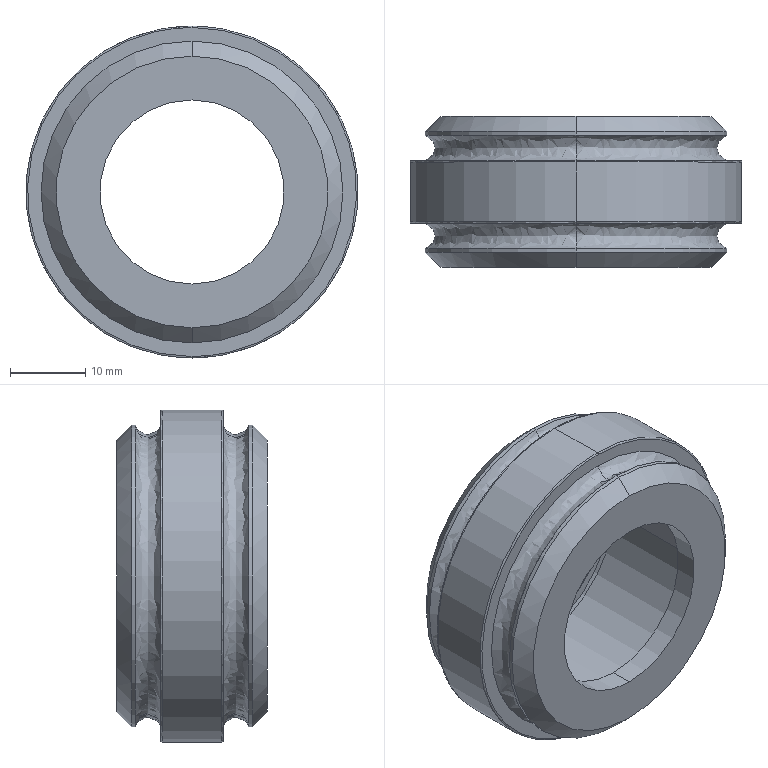Part | SolidWorks | features BaseBody 1 | 1 solid | 33 faces | box 44 x 20 x 44 mm | volume 14039 mm3 | cylinder 14 | spline 8 | plane 7 | cone 4 | commonest cylinder face diameters 28 x4 40 x4 24.4 x2 30.1 x2 44 x2
STEP:
#1=CARTESIAN_POINT('',(0.,2.5,-20.));
#2=VERTEX_POINT('',#1);
#3=CARTESIAN_POINT('',(0.,2.5,20.));
#4=VERTEX_POINT('',#3);
#5=CARTESIAN_POINT('',(0.,2.5,0.));
#6=DIRECTION('',(0.,-1.,0.));
#7=DIRECTION('',(0.,0.,1.));
#8=AXIS2_PLACEMENT_3D('',#5,#6,#7);
#9=CIRCLE('',#8,20.);
#10=EDGE_CURVE('',#2,#4,#9,.T.);
#11=ORIENTED_EDGE('',*,*,#10,.F.);
#12=CARTESIAN_POINT('',(0.,5.85,-20.));
#13=VERTEX_POINT('',#12);
#14=CARTESIAN_POINT('',(0.,4.175,-20.407));
#15=DIRECTION('',(-1.,0.,0.));
#16=DIRECTION('',(0.,0.,-1.));
#17=AXIS2_PLACEMENT_3D('',#14,#15,#16);
#18=CIRCLE('',#17,1.724);
#19=EDGE_CURVE('',#2,#13,#18,.T.);
#20=ORIENTED_EDGE('',*,*,#19,.T.);
#21=CARTESIAN_POINT('',(0.,5.85,20.));
#22=VERTEX_POINT('',#21);
#23=CARTESIAN_POINT('',(0.,5.85,0.));
#24=DIRECTION('',(0.,1.,0.));
#25=DIRECTION('',(0.,0.,1.));
#26=AXIS2_PLACEMENT_3D('',#23,#24,#25);
#27=CIRCLE('',#26,20.);
#28=EDGE_CURVE('',#22,#13,#27,.T.);
#29=ORIENTED_EDGE('',*,*,#28,.F.);
#30=CARTESIAN_POINT('',(0.,4.175,20.407));
#31=DIRECTION('',(1.,0.,0.));
#32=DIRECTION('',(0.,0.,1.));
#33=AXIS2_PLACEMENT_3D('',#30,#31,#32);
#34=CIRCLE('',#33,1.724);
#35=EDGE_CURVE('',#4,#22,#34,.T.);
#36=ORIENTED_EDGE('',*,*,#35,.F.);
#37=EDGE_LOOP('',(#11,#20,#29,#36));
#38=FACE_OUTER_BOUND('',#37,.T.);
#39=CARTESIAN_POINT('',(0.,2.5,20.));
#40=CARTESIAN_POINT('',(40.,2.5,20.));
#41=CARTESIAN_POINT('',(40.,2.5,-20.));
#42=CARTESIAN_POINT('',(0.,2.5,-20.));
#43=CARTESIAN_POINT('',(0.,3.037,17.789));
#44=CARTESIAN_POINT('',(35.578,3.037,17.789));
#45=CARTESIAN_POINT('',(35.578,3.037,-17.789));
#46=CARTESIAN_POINT('',(0.,3.037,-17.789));
#47=CARTESIAN_POINT('',(0.,5.313,17.789));
#48=CARTESIAN_POINT('',(35.578,5.313,17.789));
#49=CARTESIAN_POINT('',(35.578,5.313,-17.789));
#50=CARTESIAN_POINT('',(0.,5.313,-17.789));
#51=CARTESIAN_POINT('',(0.,5.85,20.));
#52=CARTESIAN_POINT('',(40.,5.85,20.));
#53=CARTESIAN_POINT('',(40.,5.85,-20.));
#54=CARTESIAN_POINT('',(0.,5.85,-20.));
#55=(BOUNDED_SURFACE()B_SPLINE_SURFACE(3,3,((#39,#40,#41,#42),(#43,#44,#45,#46),(#47,#48,#49,#50),(#51,#52,#53,#54)),.UNSPECIFIED.,.F.,.F.,.F.)B_SPLINE_SURFACE_WITH_KNOTS((4,4),(4,4),(0.,1.),(0.,1.),.UNSPECIFIED.)GEOMETRIC_REPRESENTATION_ITEM()RATIONAL_B_SPLINE_SURFACE(((1.,0.3333,0.3333,1.),(0.4907,0.1636,0.1636,0.4907),(0.4907,0.1636,0.1636,0.4907),(1.,0.3333,0.3333,1.)))REPRESENTATION_ITEM('')SURFACE());
#56=ADVANCED_FACE('',(#38),#55,.F.);
#57=CARTESIAN_POINT('',(0.,14.15,-20.));
#58=VERTEX_POINT('',#57);
#59=CARTESIAN_POINT('',(0.,14.15,20.));
#60=VERTEX_POINT('',#59);
#61=CARTESIAN_POINT('',(0.,14.15,0.));
#62=DIRECTION('',(0.,-1.,0.));
#63=DIRECTION('',(0.,0.,1.));
#64=AXIS2_PLACEMENT_3D('',#61,#62,#63);
#65=CIRCLE('',#64,20.);
#66=EDGE_CURVE('',#58,#60,#65,.T.);
#67=ORIENTED_EDGE('',*,*,#66,.F.);
#68=CARTESIAN_POINT('',(0.,17.5,-20.));
#69=VERTEX_POINT('',#68);
#70=CARTESIAN_POINT('',(0.,15.825,-20.407));
#71=DIRECTION('',(-1.,0.,0.));
#72=DIRECTION('',(0.,0.,-1.));
#73=AXIS2_PLACEMENT_3D('',#70,#71,#72);
#74=CIRCLE('',#73,1.724);
#75=EDGE_CURVE('',#58,#69,#74,.T.);
#76=ORIENTED_EDGE('',*,*,#75,.T.);
#77=CARTESIAN_POINT('',(0.,17.5,20.));
#78=VERTEX_POINT('',#77);
#79=CARTESIAN_POINT('',(0.,17.5,0.));
#80=DIRECTION('',(0.,1.,0.));
#81=DIRECTION('',(0.,0.,1.));
#82=AXIS2_PLACEMENT_3D('',#79,#80,#81);
#83=CIRCLE('',#82,20.);
#84=EDGE_CURVE('',#78,#69,#83,.T.);
#85=ORIENTED_EDGE('',*,*,#84,.F.);
#86=CARTESIAN_POINT('',(0.,15.825,20.407));
#87=DIRECTION('',(1.,0.,0.));
#88=DIRECTION('',(0.,0.,1.));
#89=AXIS2_PLACEMENT_3D('',#86,#87,#88);
#90=CIRCLE('',#89,1.724);
#91=EDGE_CURVE('',#60,#78,#90,.T.);
#92=ORIENTED_EDGE('',*,*,#91,.F.);
#93=EDGE_LOOP('',(#67,#76,#85,#92));
#94=FACE_OUTER_BOUND('',#93,.T.);
#95=CARTESIAN_POINT('',(0.,14.15,20.));
#96=CARTESIAN_POINT('',(40.,14.15,20.));
#97=CARTESIAN_POINT('',(40.,14.15,-20.));
#98=CARTESIAN_POINT('',(0.,14.15,-20.));
#99=CARTESIAN_POINT('',(0.,14.687,17.789));
#100=CARTESIAN_POINT('',(35.578,14.687,17.789));
#101=CARTESIAN_POINT('',(35.578,14.687,-17.789));
#102=CARTESIAN_POINT('',(0.,14.687,-17.789));
#103=CARTESIAN_POINT('',(0.,16.963,17.789));
#104=CARTESIAN_POINT('',(35.578,16.963,17.789));
#105=CARTESIAN_POINT('',(35.578,16.963,-17.789));
#106=CARTESIAN_POINT('',(0.,16.963,-17.789));
#107=CARTESIAN_POINT('',(0.,17.5,20.));
#108=CARTESIAN_POINT('',(40.,17.5,20.));
#109=CARTESIAN_POINT('',(40.,17.5,-20.));
#110=CARTESIAN_POINT('',(0.,17.5,-20.));
#111=(BOUNDED_SURFACE()B_SPLINE_SURFACE(3,3,((#95,#96,#97,#98),(#99,#100,#101,#102),(#103,#104,#105,#106),(#107,#108,#109,#110)),.UNSPECIFIED.,.F.,.F.,.T.)B_SPLINE_SURFACE_WITH_KNOTS((4,4),(4,4),(0.,1.),(0.,1.),.UNSPECIFIED.)GEOMETRIC_REPRESENTATION_ITEM()RATIONAL_B_SPLINE_SURFACE(((1.,0.3333,0.3333,1.),(0.4907,0.1636,0.1636,0.4907),(0.4907,0.1636,0.1636,0.4907),(1.,0.3333,0.3333,1.)))REPRESENTATION_ITEM('')SURFACE());
#112=ADVANCED_FACE('',(#94),#111,.F.);
#113=CARTESIAN_POINT('',(0.,6.05,22.));
#114=VERTEX_POINT('',#113);
#115=CARTESIAN_POINT('',(0.,6.05,-22.));
#116=VERTEX_POINT('',#115);
#117=CARTESIAN_POINT('',(0.,6.05,0.));
#118=DIRECTION('',(0.,-1.,0.));
#119=DIRECTION('',(0.,0.,1.));
#120=AXIS2_PLACEMENT_3D('',#117,#118,#119);
#121=CIRCLE('',#120,22.);
#122=EDGE_CURVE('',#114,#116,#121,.T.);
#123=ORIENTED_EDGE('',*,*,#122,.T.);
#124=CARTESIAN_POINT('',(0.,5.85,-21.8));
#125=VERTEX_POINT('',#124);
#126=CARTESIAN_POINT('',(0.,6.05,-21.8));
#127=DIRECTION('',(-1.,0.,0.));
#128=DIRECTION('',(0.,0.,-1.));
#129=AXIS2_PLACEMENT_3D('',#126,#127,#128);
#130=CIRCLE('',#129,0.2);
#131=EDGE_CURVE('',#116,#125,#130,.T.);
#132=ORIENTED_EDGE('',*,*,#131,.T.);
#133=CARTESIAN_POINT('',(0.,5.85,21.8));
#134=VERTEX_POINT('',#133);
#135=CARTESIAN_POINT('',(0.,5.85,-21.8));
#136=CARTESIAN_POINT('',(-43.6,5.85,-21.8));
#137=CARTESIAN_POINT('',(-43.6,5.85,21.8));
#138=CARTESIAN_POINT('',(0.,5.85,21.8));
#139=(BOUNDED_CURVE()B_SPLINE_CURVE(3,(#135,#136,#137,#138),.UNSPECIFIED.,.F.,.F.)B_SPLINE_CURVE_WITH_KNOTS((4,4),(0.,1.),.UNSPECIFIED.)CURVE()GEOMETRIC_REPRESENTATION_ITEM()RATIONAL_B_SPLINE_CURVE((1.,0.3333,0.3333,1.))REPRESENTATION_ITEM(''));
#140=EDGE_CURVE('',#125,#134,#139,.T.);
#141=ORIENTED_EDGE('',*,*,#140,.T.);
#142=CARTESIAN_POINT('',(0.,6.05,21.8));
#143=DIRECTION('',(1.,0.,0.));
#144=DIRECTION('',(0.,0.,1.));
#145=AXIS2_PLACEMENT_3D('',#142,#143,#144);
#146=CIRCLE('',#145,0.2);
#147=EDGE_CURVE('',#114,#134,#146,.T.);
#148=ORIENTED_EDGE('',*,*,#147,.F.);
#149=EDGE_LOOP('',(#123,#132,#141,#148));
#150=FACE_OUTER_BOUND('',#149,.T.);
#151=CARTESIAN_POINT('',(0.,6.05,-22.));
#152=CARTESIAN_POINT('',(-44.,6.05,-22.));
#153=CARTESIAN_POINT('',(-44.,6.05,22.));
#154=CARTESIAN_POINT('',(0.,6.05,22.));
#155=CARTESIAN_POINT('',(0.,5.933,-22.));
#156=CARTESIAN_POINT('',(-44.,5.933,-22.));
#157=CARTESIAN_POINT('',(-44.,5.933,22.));
#158=CARTESIAN_POINT('',(0.,5.933,22.));
#159=CARTESIAN_POINT('',(0.,5.85,-21.917));
#160=CARTESIAN_POINT('',(-43.834,5.85,-21.917));
#161=CARTESIAN_POINT('',(-43.834,5.85,21.917));
#162=CARTESIAN_POINT('',(0.,5.85,21.917));
#163=CARTESIAN_POINT('',(0.,5.85,-21.8));
#164=CARTESIAN_POINT('',(-43.6,5.85,-21.8));
#165=CARTESIAN_POINT('',(-43.6,5.85,21.8));
#166=CARTESIAN_POINT('',(0.,5.85,21.8));
#167=(BOUNDED_SURFACE()B_SPLINE_SURFACE(3,3,((#151,#152,#153,#154),(#155,#156,#157,#158),(#159,#160,#161,#162),(#163,#164,#165,#166)),.UNSPECIFIED.,.F.,.F.,.F.)B_SPLINE_SURFACE_WITH_KNOTS((4,4),(4,4),(0.,1.),(0.,1.),.UNSPECIFIED.)GEOMETRIC_REPRESENTATION_ITEM()RATIONAL_B_SPLINE_SURFACE(((1.,0.3333,0.3333,1.),(0.8047,0.2682,0.2682,0.8047),(0.8047,0.2682,0.2682,0.8047),(1.,0.3333,0.3333,1.)))REPRESENTATION_ITEM('')SURFACE());
#168=ADVANCED_FACE('',(#150),#167,.T.);
#169=CARTESIAN_POINT('',(0.,13.95,22.));
#170=VERTEX_POINT('',#169);
#171=CARTESIAN_POINT('',(0.,13.95,-22.));
#172=VERTEX_POINT('',#171);
#173=CARTESIAN_POINT('',(0.,13.95,0.));
#174=DIRECTION('',(0.,-1.,0.));
#175=DIRECTION('',(0.,0.,1.));
#176=AXIS2_PLACEMENT_3D('',#173,#174,#175);
#177=CIRCLE('',#176,22.);
#178=EDGE_CURVE('',#170,#172,#177,.T.);
#179=ORIENTED_EDGE('',*,*,#178,.F.);
#180=CARTESIAN_POINT('',(0.,14.15,21.8));
#181=VERTEX_POINT('',#180);
#182=CARTESIAN_POINT('',(0.,13.95,21.8));
#183=DIRECTION('',(-1.,0.,0.));
#184=DIRECTION('',(0.,0.,1.));
#185=AXIS2_PLACEMENT_3D('',#182,#183,#184);
#186=CIRCLE('',#185,0.2);
#187=EDGE_CURVE('',#170,#181,#186,.T.);
#188=ORIENTED_EDGE('',*,*,#187,.T.);
#189=CARTESIAN_POINT('',(0.,14.15,-21.8));
#190=VERTEX_POINT('',#189);
#191=CARTESIAN_POINT('',(0.,14.15,21.8));
#192=CARTESIAN_POINT('',(-43.6,14.15,21.8));
#193=CARTESIAN_POINT('',(-43.6,14.15,-21.8));
#194=CARTESIAN_POINT('',(0.,14.15,-21.8));
#195=(BOUNDED_CURVE()B_SPLINE_CURVE(3,(#191,#192,#193,#194),.UNSPECIFIED.,.F.,.F.)B_SPLINE_CURVE_WITH_KNOTS((4,4),(0.,1.),.UNSPECIFIED.)CURVE()GEOMETRIC_REPRESENTATION_ITEM()RATIONAL_B_SPLINE_CURVE((1.,0.3333,0.3333,1.))REPRESENTATION_ITEM(''));
#196=EDGE_CURVE('',#181,#190,#195,.T.);
#197=ORIENTED_EDGE('',*,*,#196,.T.);
#198=CARTESIAN_POINT('',(0.,13.95,-21.8));
#199=DIRECTION('',(1.,0.,0.));
#200=DIRECTION('',(0.,0.,-1.));
#201=AXIS2_PLACEMENT_3D('',#198,#199,#200);
#202=CIRCLE('',#201,0.2);
#203=EDGE_CURVE('',#172,#190,#202,.T.);
#204=ORIENTED_EDGE('',*,*,#203,.F.);
#205=EDGE_LOOP('',(#179,#188,#197,#204));
#206=FACE_OUTER_BOUND('',#205,.T.);
#207=CARTESIAN_POINT('',(0.,13.95,22.));
#208=CARTESIAN_POINT('',(-44.,13.95,22.));
#209=CARTESIAN_POINT('',(-44.,13.95,-22.));
#210=CARTESIAN_POINT('',(0.,13.95,-22.));
#211=CARTESIAN_POINT('',(0.,14.067,22.));
#212=CARTESIAN_POINT('',(-44.,14.067,22.));
#213=CARTESIAN_POINT('',(-44.,14.067,-22.));
#214=CARTESIAN_POINT('',(0.,14.067,-22.));
#215=CARTESIAN_POINT('',(0.,14.15,21.917));
#216=CARTESIAN_POINT('',(-43.834,14.15,21.917));
#217=CARTESIAN_POINT('',(-43.834,14.15,-21.917));
#218=CARTESIAN_POINT('',(0.,14.15,-21.917));
#219=CARTESIAN_POINT('',(0.,14.15,21.8));
#220=CARTESIAN_POINT('',(-43.6,14.15,21.8));
#221=CARTESIAN_POINT('',(-43.6,14.15,-21.8));
#222=CARTESIAN_POINT('',(0.,14.15,-21.8));
#223=(BOUNDED_SURFACE()B_SPLINE_SURFACE(3,3,((#207,#208,#209,#210),(#211,#212,#213,#214),(#215,#216,#217,#218),(#219,#220,#221,#222)),.UNSPECIFIED.,.F.,.F.,.T.)B_SPLINE_SURFACE_WITH_KNOTS((4,4),(4,4),(0.,1.),(0.,1.),.UNSPECIFIED.)GEOMETRIC_REPRESENTATION_ITEM()RATIONAL_B_SPLINE_SURFACE(((1.,0.3333,0.3333,1.),(0.8047,0.2682,0.2682,0.8047),(0.8047,0.2682,0.2682,0.8047),(1.,0.3333,0.3333,1.)))REPRESENTATION_ITEM('')SURFACE());
#224=ADVANCED_FACE('',(#206),#223,.T.);
#225=CARTESIAN_POINT('',(14.,3.,0.));
#226=VERTEX_POINT('',#225);
#227=CARTESIAN_POINT('',(-14.,3.,0.));
#228=VERTEX_POINT('',#227);
#229=CARTESIAN_POINT('',(0.,3.,0.));
#230=DIRECTION('',(0.,1.,0.));
#231=DIRECTION('',(-1.,0.,0.));
#232=AXIS2_PLACEMENT_3D('',#229,#230,#231);
#233=CIRCLE('',#232,14.);
#234=EDGE_CURVE('',#226,#228,#233,.T.);
#235=ORIENTED_EDGE('',*,*,#234,.F.);
#236=CARTESIAN_POINT('',(14.,17.,0.));
#237=VERTEX_POINT('',#236);
#238=CARTESIAN_POINT('',(14.,3.,0.));
#239=DIRECTION('',(0.,1.,0.));
#240=VECTOR('',#239,1000.);
#241=LINE('',#238,#240);
#242=EDGE_CURVE('',#226,#237,#241,.T.);
#243=ORIENTED_EDGE('',*,*,#242,.T.);
#244=CARTESIAN_POINT('',(-14.,17.,0.));
#245=VERTEX_POINT('',#244);
#246=CARTESIAN_POINT('',(0.,17.,0.));
#247=DIRECTION('',(0.,-1.,0.));
#248=DIRECTION('',(-1.,0.,0.));
#249=AXIS2_PLACEMENT_3D('',#246,#247,#248);
#250=CIRCLE('',#249,14.);
#251=EDGE_CURVE('',#245,#237,#250,.T.);
#252=ORIENTED_EDGE('',*,*,#251,.F.);
#253=CARTESIAN_POINT('',(-14.,3.,0.));
#254=DIRECTION('',(0.,1.,0.));
#255=VECTOR('',#254,1000.);
#256=LINE('',#253,#255);
#257=EDGE_CURVE('',#228,#245,#256,.T.);
#258=ORIENTED_EDGE('',*,*,#257,.F.);
#259=EDGE_LOOP('',(#235,#243,#252,#258));
#260=FACE_OUTER_BOUND('',#259,.T.);
#261=CARTESIAN_POINT('',(0.,3.,0.));
#262=DIRECTION('',(0.,1.,0.));
#263=DIRECTION('',(-1.,0.,0.));
#264=AXIS2_PLACEMENT_3D('',#261,#262,#263);
#265=CYLINDRICAL_SURFACE('',#264,14.);
#266=ADVANCED_FACE('',(#260),#265,.F.);
#267=CARTESIAN_POINT('',(0.,3.,12.2));
#268=VERTEX_POINT('',#267);
#269=CARTESIAN_POINT('',(0.,3.,-12.2));
#270=VERTEX_POINT('',#269);
#271=CARTESIAN_POINT('',(0.,3.,0.));
#272=DIRECTION('',(0.,-1.,0.));
#273=DIRECTION('',(0.,0.,-1.));
#274=AXIS2_PLACEMENT_3D('',#271,#272,#273);
#275=CIRCLE('',#274,12.2);
#276=EDGE_CURVE('',#268,#270,#275,.T.);
#277=ORIENTED_EDGE('',*,*,#276,.F.);
#278=CARTESIAN_POINT('',(0.,0.,12.2));
#279=VERTEX_POINT('',#278);
#280=CARTESIAN_POINT('',(0.,20.,12.2));
#281=DIRECTION('',(0.,-1.,0.));
#282=VECTOR('',#281,1000.);
#283=LINE('',#280,#282);
#284=EDGE_CURVE('',#268,#279,#283,.T.);
#285=ORIENTED_EDGE('',*,*,#284,.T.);
#286=CARTESIAN_POINT('',(0.,0.,-12.2));
#287=VERTEX_POINT('',#286);
#288=CARTESIAN_POINT('',(0.,0.,0.));
#289=DIRECTION('',(0.,1.,0.));
#290=DIRECTION('',(0.,0.,-1.));
#291=AXIS2_PLACEMENT_3D('',#288,#289,#290);
#292=CIRCLE('',#291,12.2);
#293=EDGE_CURVE('',#287,#279,#292,.T.);
#294=ORIENTED_EDGE('',*,*,#293,.F.);
#295=CARTESIAN_POINT('',(0.,20.,-12.2));
#296=DIRECTION('',(0.,-1.,0.));
#297=VECTOR('',#296,1000.);
#298=LINE('',#295,#297);
#299=EDGE_CURVE('',#270,#287,#298,.T.);
#300=ORIENTED_EDGE('',*,*,#299,.F.);
#301=EDGE_LOOP('',(#277,#285,#294,#300));
#302=FACE_OUTER_BOUND('',#301,.T.);
#303=CARTESIAN_POINT('',(0.,20.,0.));
#304=DIRECTION('',(0.,-1.,0.));
#305=DIRECTION('',(0.,0.,-1.));
#306=AXIS2_PLACEMENT_3D('',#303,#304,#305);
#307=CYLINDRICAL_SURFACE('',#306,12.2);
#308=ADVANCED_FACE('',(#302),#307,.F.);
#309=CARTESIAN_POINT('',(-15.05,18.3,0.));
#310=VERTEX_POINT('',#309);
#311=CARTESIAN_POINT('',(15.05,18.3,0.));
#312=VERTEX_POINT('',#311);
#313=CARTESIAN_POINT('',(0.,18.3,0.));
#314=DIRECTION('',(0.,-1.,0.));
#315=DIRECTION('',(1.,0.,0.));
#316=AXIS2_PLACEMENT_3D('',#313,#314,#315);
#317=CIRCLE('',#316,15.05);
#318=EDGE_CURVE('',#310,#312,#317,.T.);
#319=ORIENTED_EDGE('',*,*,#318,.F.);
#320=CARTESIAN_POINT('',(-15.05,17.,0.));
#321=VERTEX_POINT('',#320);
#322=CARTESIAN_POINT('',(-15.05,18.3,0.));
#323=DIRECTION('',(0.,-1.,0.));
#324=VECTOR('',#323,1000.);
#325=LINE('',#322,#324);
#326=EDGE_CURVE('',#310,#321,#325,.T.);
#327=ORIENTED_EDGE('',*,*,#326,.T.);
#328=CARTESIAN_POINT('',(15.05,17.,0.));
#329=VERTEX_POINT('',#328);
#330=CARTESIAN_POINT('',(0.,17.,0.));
#331=DIRECTION('',(0.,1.,0.));
#332=DIRECTION('',(1.,0.,0.));
#333=AXIS2_PLACEMENT_3D('',#330,#331,#332);
#334=CIRCLE('',#333,15.05);
#335=EDGE_CURVE('',#329,#321,#334,.T.);
#336=ORIENTED_EDGE('',*,*,#335,.F.);
#337=CARTESIAN_POINT('',(15.05,18.3,0.));
#338=DIRECTION('',(0.,-1.,0.));
#339=VECTOR('',#338,1000.);
#340=LINE('',#337,#339);
#341=EDGE_CURVE('',#312,#329,#340,.T.);
#342=ORIENTED_EDGE('',*,*,#341,.F.);
#343=EDGE_LOOP('',(#319,#327,#336,#342));
#344=FACE_OUTER_BOUND('',#343,.T.);
#345=CARTESIAN_POINT('',(0.,18.3,0.));
#346=DIRECTION('',(0.,-1.,0.));
#347=DIRECTION('',(1.,0.,0.));
#348=AXIS2_PLACEMENT_3D('',#345,#346,#347);
#349=CYLINDRICAL_SURFACE('',#348,15.05);
#350=ADVANCED_FACE('',(#344),#349,.F.);
#351=CARTESIAN_POINT('',(0.,0.,18.));
#352=VERTEX_POINT('',#351);
#353=CARTESIAN_POINT('',(0.,0.,-18.));
#354=VERTEX_POINT('',#353);
#355=CARTESIAN_POINT('',(0.,0.,0.));
#356=DIRECTION('',(0.,1.,0.));
#357=DIRECTION('',(0.,0.,1.));
#358=AXIS2_PLACEMENT_3D('',#355,#356,#357);
#359=CIRCLE('',#358,18.);
#360=EDGE_CURVE('',#352,#354,#359,.T.);
#361=ORIENTED_EDGE('',*,*,#360,.T.);
#362=CARTESIAN_POINT('',(0.,2.,-20.));
#363=VERTEX_POINT('',#362);
#364=CARTESIAN_POINT('',(0.,2.,-20.));
#365=DIRECTION('',(0.,0.7071,-0.7071));
#366=VECTOR('',#365,1000.);
#367=LINE('',#364,#366);
#368=EDGE_CURVE('',#354,#363,#367,.T.);
#369=ORIENTED_EDGE('',*,*,#368,.T.);
#370=CARTESIAN_POINT('',(0.,2.,20.));
#371=VERTEX_POINT('',#370);
#372=CARTESIAN_POINT('',(0.,2.,0.));
#373=DIRECTION('',(0.,-1.,0.));
#374=DIRECTION('',(0.,0.,1.));
#375=AXIS2_PLACEMENT_3D('',#372,#373,#374);
#376=CIRCLE('',#375,20.);
#377=EDGE_CURVE('',#363,#371,#376,.T.);
#378=ORIENTED_EDGE('',*,*,#377,.T.);
#379=CARTESIAN_POINT('',(0.,2.,20.));
#380=DIRECTION('',(0.,0.7071,0.7071));
#381=VECTOR('',#380,1000.);
#382=LINE('',#379,#381);
#383=EDGE_CURVE('',#352,#371,#382,.T.);
#384=ORIENTED_EDGE('',*,*,#383,.F.);
#385=EDGE_LOOP('',(#361,#369,#378,#384));
#386=FACE_OUTER_BOUND('',#385,.T.);
#387=CARTESIAN_POINT('',(0.,2.,0.));
#388=DIRECTION('',(0.,1.,0.));
#389=DIRECTION('',(0.,0.,1.));
#390=AXIS2_PLACEMENT_3D('',#387,#388,#389);
#391=CONICAL_SURFACE('',#390,20.,0.7854);
#392=ADVANCED_FACE('',(#386),#391,.T.);
#393=CARTESIAN_POINT('',(-14.,18.3,0.));
#394=VERTEX_POINT('',#393);
#395=CARTESIAN_POINT('',(14.,18.3,0.));
#396=VERTEX_POINT('',#395);
#397=CARTESIAN_POINT('',(0.,18.3,0.));
#398=DIRECTION('',(0.,-1.,0.));
#399=DIRECTION('',(-1.,0.,0.));
#400=AXIS2_PLACEMENT_3D('',#397,#398,#399);
#401=CIRCLE('',#400,14.);
#402=EDGE_CURVE('',#394,#396,#401,.T.);
#403=ORIENTED_EDGE('',*,*,#402,.T.);
#404=CARTESIAN_POINT('',(14.,20.,0.));
#405=VERTEX_POINT('',#404);
#406=CARTESIAN_POINT('',(14.,3.,0.));
#407=DIRECTION('',(0.,1.,0.));
#408=VECTOR('',#407,1000.);
#409=LINE('',#406,#408);
#410=EDGE_CURVE('',#396,#405,#409,.T.);
#411=ORIENTED_EDGE('',*,*,#410,.T.);
#412=CARTESIAN_POINT('',(-14.,20.,0.));
#413=VERTEX_POINT('',#412);
#414=CARTESIAN_POINT('',(0.,20.,0.));
#415=DIRECTION('',(0.,-1.,0.));
#416=DIRECTION('',(-1.,0.,0.));
#417=AXIS2_PLACEMENT_3D('',#414,#415,#416);
#418=CIRCLE('',#417,14.);
#419=EDGE_CURVE('',#413,#405,#418,.T.);
#420=ORIENTED_EDGE('',*,*,#419,.F.);
#421=CARTESIAN_POINT('',(-14.,3.,0.));
#422=DIRECTION('',(0.,1.,0.));
#423=VECTOR('',#422,1000.);
#424=LINE('',#421,#423);
#425=EDGE_CURVE('',#394,#413,#424,.T.);
#426=ORIENTED_EDGE('',*,*,#425,.F.);
#427=EDGE_LOOP('',(#403,#411,#420,#426));
#428=FACE_OUTER_BOUND('',#427,.T.);
#429=CARTESIAN_POINT('',(0.,3.,0.));
#430=DIRECTION('',(0.,1.,0.));
#431=DIRECTION('',(-1.,0.,0.));
#432=AXIS2_PLACEMENT_3D('',#429,#430,#431);
#433=CYLINDRICAL_SURFACE('',#432,14.);
#434=ADVANCED_FACE('',(#428),#433,.F.);
#435=ORIENTED_EDGE('',*,*,#377,.F.);
#436=CARTESIAN_POINT('',(0.,20.,-20.));
#437=DIRECTION('',(0.,1.,0.));
#438=VECTOR('',#437,1000.);
#439=LINE('',#436,#438);
#440=EDGE_CURVE('',#363,#2,#439,.T.);
#441=ORIENTED_EDGE('',*,*,#440,.T.);
#442=ORIENTED_EDGE('',*,*,#10,.T.);
#443=CARTESIAN_POINT('',(0.,20.,20.));
#444=DIRECTION('',(0.,1.,0.));
#445=VECTOR('',#444,1000.);
#446=LINE('',#443,#445);
#447=EDGE_CURVE('',#371,#4,#446,.T.);
#448=ORIENTED_EDGE('',*,*,#447,.F.);
#449=EDGE_LOOP('',(#435,#441,#442,#448));
#450=FACE_OUTER_BOUND('',#449,.T.);
#451=CARTESIAN_POINT('',(0.,20.,0.));
#452=DIRECTION('',(0.,1.,0.));
#453=DIRECTION('',(0.,0.,1.));
#454=AXIS2_PLACEMENT_3D('',#451,#452,#453);
#455=CYLINDRICAL_SURFACE('',#454,20.);
#456=ADVANCED_FACE('',(#450),#455,.T.);
#457=CARTESIAN_POINT('',(0.,20.,-18.));
#458=VERTEX_POINT('',#457);
#459=CARTESIAN_POINT('',(0.,20.,18.));
#460=VERTEX_POINT('',#459);
#461=CARTESIAN_POINT('',(0.,20.,0.));
#462=DIRECTION('',(0.,-1.,0.));
#463=DIRECTION('',(0.,0.,-1.));
#464=AXIS2_PLACEMENT_3D('',#461,#462,#463);
#465=CIRCLE('',#464,18.);
#466=EDGE_CURVE('',#458,#460,#465,.T.);
#467=ORIENTED_EDGE('',*,*,#466,.T.);
#468=CARTESIAN_POINT('',(0.,18.,20.));
#469=VERTEX_POINT('',#468);
#470=CARTESIAN_POINT('',(0.,18.,20.));
#471=DIRECTION('',(0.,-0.7071,0.7071));
#472=VECTOR('',#471,1000.);
#473=LINE('',#470,#472);
#474=EDGE_CURVE('',#460,#469,#473,.T.);
#475=ORIENTED_EDGE('',*,*,#474,.T.);
#476=CARTESIAN_POINT('',(0.,18.,-20.));
#477=VERTEX_POINT('',#476);
#478=CARTESIAN_POINT('',(0.,18.,0.));
#479=DIRECTION('',(0.,1.,0.));
#480=DIRECTION('',(0.,0.,-1.));
#481=AXIS2_PLACEMENT_3D('',#478,#479,#480);
#482=CIRCLE('',#481,20.);
#483=EDGE_CURVE('',#469,#477,#482,.T.);
#484=ORIENTED_EDGE('',*,*,#483,.T.);
#485=CARTESIAN_POINT('',(0.,18.,-20.));
#486=DIRECTION('',(0.,-0.7071,-0.7071));
#487=VECTOR('',#486,1000.);
#488=LINE('',#485,#487);
#489=EDGE_CURVE('',#458,#477,#488,.T.);
#490=ORIENTED_EDGE('',*,*,#489,.F.);
#491=EDGE_LOOP('',(#467,#475,#484,#490));
#492=FACE_OUTER_BOUND('',#491,.T.);
#493=CARTESIAN_POINT('',(0.,18.,0.));
#494=DIRECTION('',(0.,-1.,0.));
#495=DIRECTION('',(0.,0.,-1.));
#496=AXIS2_PLACEMENT_3D('',#493,#494,#495);
#497=CONICAL_SURFACE('',#496,20.,0.7854);
#498=ADVANCED_FACE('',(#492),#497,.T.);
#499=ORIENTED_EDGE('',*,*,#84,.T.);
#500=CARTESIAN_POINT('',(0.,20.,-20.));
#501=DIRECTION('',(0.,1.,0.));
#502=VECTOR('',#501,1000.);
#503=LINE('',#500,#502);
#504=EDGE_CURVE('',#69,#477,#503,.T.);
#505=ORIENTED_EDGE('',*,*,#504,.T.);
#506=ORIENTED_EDGE('',*,*,#483,.F.);
#507=CARTESIAN_POINT('',(0.,20.,20.));
#508=DIRECTION('',(0.,1.,0.));
#509=VECTOR('',#508,1000.);
#510=LINE('',#507,#509);
#511=EDGE_CURVE('',#78,#469,#510,.T.);
#512=ORIENTED_EDGE('',*,*,#511,.F.);
#513=EDGE_LOOP('',(#499,#505,#506,#512));
#514=FACE_OUTER_BOUND('',#513,.T.);
#515=CARTESIAN_POINT('',(0.,20.,0.));
#516=DIRECTION('',(0.,1.,0.));
#517=DIRECTION('',(0.,0.,1.));
#518=AXIS2_PLACEMENT_3D('',#515,#516,#517);
#519=CYLINDRICAL_SURFACE('',#518,20.);
#520=ADVANCED_FACE('',(#514),#519,.T.);
#521=CARTESIAN_POINT('',(0.,6.05,0.));
#522=DIRECTION('',(0.,-1.,0.));
#523=DIRECTION('',(0.,0.,1.));
#524=AXIS2_PLACEMENT_3D('',#521,#522,#523);
#525=CIRCLE('',#524,22.);
#526=EDGE_CURVE('',#116,#114,#525,.T.);
#527=ORIENTED_EDGE('',*,*,#526,.F.);
#528=CARTESIAN_POINT('',(0.,20.,-22.));
#529=DIRECTION('',(0.,1.,0.));
#530=VECTOR('',#529,1000.);
#531=LINE('',#528,#530);
#532=EDGE_CURVE('',#116,#172,#531,.T.);
#533=ORIENTED_EDGE('',*,*,#532,.T.);
#534=CARTESIAN_POINT('',(0.,13.95,0.));
#535=DIRECTION('',(0.,-1.,0.));
#536=DIRECTION('',(0.,0.,1.));
#537=AXIS2_PLACEMENT_3D('',#534,#535,#536);
#538=CIRCLE('',#537,22.);
#539=EDGE_CURVE('',#172,#170,#538,.T.);
#540=ORIENTED_EDGE('',*,*,#539,.T.);
#541=CARTESIAN_POINT('',(0.,20.,22.));
#542=DIRECTION('',(0.,1.,0.));
#543=VECTOR('',#542,1000.);
#544=LINE('',#541,#543);
#545=EDGE_CURVE('',#114,#170,#544,.T.);
#546=ORIENTED_EDGE('',*,*,#545,.F.);
#547=EDGE_LOOP('',(#527,#533,#540,#546));
#548=FACE_OUTER_BOUND('',#547,.T.);
#549=CARTESIAN_POINT('',(0.,20.,0.));
#550=DIRECTION('',(0.,1.,0.));
#551=DIRECTION('',(0.,0.,1.));
#552=AXIS2_PLACEMENT_3D('',#549,#550,#551);
#553=CYLINDRICAL_SURFACE('',#552,22.);
#554=ADVANCED_FACE('',(#548),#553,.T.);
#555=ORIENTED_EDGE('',*,*,#242,.F.);
#556=CARTESIAN_POINT('',(0.,3.,0.));
#557=DIRECTION('',(0.,1.,0.));
#558=DIRECTION('',(-1.,0.,0.));
#559=AXIS2_PLACEMENT_3D('',#556,#557,#558);
#560=CIRCLE('',#559,14.);
#561=EDGE_CURVE('',#228,#226,#560,.T.);
#562=ORIENTED_EDGE('',*,*,#561,.F.);
#563=ORIENTED_EDGE('',*,*,#257,.T.);
#564=CARTESIAN_POINT('',(0.,17.,0.));
#565=DIRECTION('',(0.,-1.,0.));
#566=DIRECTION('',(-1.,0.,0.));
#567=AXIS2_PLACEMENT_3D('',#564,#565,#566);
#568=CIRCLE('',#567,14.);
#569=EDGE_CURVE('',#237,#245,#568,.T.);
#570=ORIENTED_EDGE('',*,*,#569,.F.);
#571=EDGE_LOOP('',(#555,#562,#563,#570));
#572=FACE_OUTER_BOUND('',#571,.T.);
#573=CARTESIAN_POINT('',(0.,3.,0.));
#574=DIRECTION('',(0.,1.,0.));
#575=DIRECTION('',(-1.,0.,0.));
#576=AXIS2_PLACEMENT_3D('',#573,#574,#575);
#577=CYLINDRICAL_SURFACE('',#576,14.);
#578=ADVANCED_FACE('',(#572),#577,.F.);
#579=ORIENTED_EDGE('',*,*,#561,.T.);
#580=ORIENTED_EDGE('',*,*,#234,.T.);
#581=EDGE_LOOP('',(#579,#580));
#582=FACE_OUTER_BOUND('',#581,.T.);
#583=CARTESIAN_POINT('',(0.,3.,0.));
#584=DIRECTION('',(0.,-1.,0.));
#585=DIRECTION('',(0.,0.,-1.));
#586=AXIS2_PLACEMENT_3D('',#583,#584,#585);
#587=CIRCLE('',#586,12.2);
#588=EDGE_CURVE('',#270,#268,#587,.T.);
#589=ORIENTED_EDGE('',*,*,#588,.T.);
#590=ORIENTED_EDGE('',*,*,#276,.T.);
#591=EDGE_LOOP('',(#589,#590));
#592=FACE_BOUND('',#591,.T.);
#593=CARTESIAN_POINT('',(0.,3.,0.));
#594=DIRECTION('',(0.,1.,0.));
#595=DIRECTION('',(-1.,0.,0.));
#596=AXIS2_PLACEMENT_3D('',#593,#594,#595);
#597=PLANE('',#596);
#598=ADVANCED_FACE('',(#582,#592),#597,.T.);
#599=ORIENTED_EDGE('',*,*,#251,.T.);
#600=ORIENTED_EDGE('',*,*,#569,.T.);
#601=EDGE_LOOP('',(#599,#600));
#602=FACE_BOUND('',#601,.T.);
#603=ORIENTED_EDGE('',*,*,#335,.T.);
#604=CARTESIAN_POINT('',(0.,17.,0.));
#605=DIRECTION('',(0.,1.,0.));
#606=DIRECTION('',(1.,0.,0.));
#607=AXIS2_PLACEMENT_3D('',#604,#605,#606);
#608=CIRCLE('',#607,15.05);
#609=EDGE_CURVE('',#321,#329,#608,.T.);
#610=ORIENTED_EDGE('',*,*,#609,.T.);
#611=EDGE_LOOP('',(#603,#610));
#612=FACE_OUTER_BOUND('',#611,.T.);
#613=CARTESIAN_POINT('',(0.,17.,0.));
#614=DIRECTION('',(0.,1.,0.));
#615=DIRECTION('',(-1.,0.,0.));
#616=AXIS2_PLACEMENT_3D('',#613,#614,#615);
#617=PLANE('',#616);
#618=ADVANCED_FACE('',(#602,#612),#617,.T.);
#619=ORIENTED_EDGE('',*,*,#284,.F.);
#620=ORIENTED_EDGE('',*,*,#588,.F.);
#621=ORIENTED_EDGE('',*,*,#299,.T.);
#622=CARTESIAN_POINT('',(0.,0.,0.));
#623=DIRECTION('',(0.,1.,0.));
#624=DIRECTION('',(0.,0.,-1.));
#625=AXIS2_PLACEMENT_3D('',#622,#623,#624);
#626=CIRCLE('',#625,12.2);
#627=EDGE_CURVE('',#279,#287,#626,.T.);
#628=ORIENTED_EDGE('',*,*,#627,.F.);
#629=EDGE_LOOP('',(#619,#620,#621,#628));
#630=FACE_OUTER_BOUND('',#629,.T.);
#631=CARTESIAN_POINT('',(0.,20.,0.));
#632=DIRECTION('',(0.,-1.,0.));
#633=DIRECTION('',(0.,0.,-1.));
#634=AXIS2_PLACEMENT_3D('',#631,#632,#633);
#635=CYLINDRICAL_SURFACE('',#634,12.2);
#636=ADVANCED_FACE('',(#630),#635,.F.);
#637=ORIENTED_EDGE('',*,*,#326,.F.);
#638=CARTESIAN_POINT('',(0.,18.3,0.));
#639=DIRECTION('',(0.,-1.,0.));
#640=DIRECTION('',(1.,0.,0.));
#641=AXIS2_PLACEMENT_3D('',#638,#639,#640);
#642=CIRCLE('',#641,15.05);
#643=EDGE_CURVE('',#312,#310,#642,.T.);
#644=ORIENTED_EDGE('',*,*,#643,.F.);
#645=ORIENTED_EDGE('',*,*,#341,.T.);
#646=ORIENTED_EDGE('',*,*,#609,.F.);
#647=EDGE_LOOP('',(#637,#644,#645,#646));
#648=FACE_OUTER_BOUND('',#647,.T.);
#649=CARTESIAN_POINT('',(0.,18.3,0.));
#650=DIRECTION('',(0.,-1.,0.));
#651=DIRECTION('',(1.,0.,0.));
#652=AXIS2_PLACEMENT_3D('',#649,#650,#651);
#653=CYLINDRICAL_SURFACE('',#652,15.05);
#654=ADVANCED_FACE('',(#648),#653,.F.);
#655=ORIENTED_EDGE('',*,*,#360,.F.);
#656=CARTESIAN_POINT('',(0.,0.,0.));
#657=DIRECTION('',(0.,1.,0.));
#658=DIRECTION('',(0.,0.,1.));
#659=AXIS2_PLACEMENT_3D('',#656,#657,#658);
#660=CIRCLE('',#659,18.);
#661=EDGE_CURVE('',#354,#352,#660,.T.);
#662=ORIENTED_EDGE('',*,*,#661,.F.);
#663=EDGE_LOOP('',(#655,#662));
#664=FACE_OUTER_BOUND('',#663,.T.);
#665=ORIENTED_EDGE('',*,*,#293,.T.);
#666=ORIENTED_EDGE('',*,*,#627,.T.);
#667=EDGE_LOOP('',(#665,#666));
#668=FACE_BOUND('',#667,.T.);
#669=CARTESIAN_POINT('',(0.,0.,0.));
#670=DIRECTION('',(0.,1.,0.));
#671=DIRECTION('',(0.,0.,1.));
#672=AXIS2_PLACEMENT_3D('',#669,#670,#671);
#673=PLANE('',#672);
#674=ADVANCED_FACE('',(#664,#668),#673,.F.);
#675=ORIENTED_EDGE('',*,*,#402,.F.);
#676=CARTESIAN_POINT('',(0.,18.3,0.));
#677=DIRECTION('',(0.,-1.,0.));
#678=DIRECTION('',(-1.,0.,0.));
#679=AXIS2_PLACEMENT_3D('',#676,#677,#678);
#680=CIRCLE('',#679,14.);
#681=EDGE_CURVE('',#396,#394,#680,.T.);
#682=ORIENTED_EDGE('',*,*,#681,.F.);
#683=EDGE_LOOP('',(#675,#682));
#684=FACE_BOUND('',#683,.T.);
#685=ORIENTED_EDGE('',*,*,#643,.T.);
#686=ORIENTED_EDGE('',*,*,#318,.T.);
#687=EDGE_LOOP('',(#685,#686));
#688=FACE_OUTER_BOUND('',#687,.T.);
#689=CARTESIAN_POINT('',(0.,18.3,0.));
#690=DIRECTION('',(0.,1.,0.));
#691=DIRECTION('',(-1.,0.,0.));
#692=AXIS2_PLACEMENT_3D('',#689,#690,#691);
#693=PLANE('',#692);
#694=ADVANCED_FACE('',(#684,#688),#693,.F.);
#695=ORIENTED_EDGE('',*,*,#368,.F.);
#696=ORIENTED_EDGE('',*,*,#661,.T.);
#697=ORIENTED_EDGE('',*,*,#383,.T.);
#698=CARTESIAN_POINT('',(0.,2.,0.));
#699=DIRECTION('',(0.,-1.,0.));
#700=DIRECTION('',(0.,0.,1.));
#701=AXIS2_PLACEMENT_3D('',#698,#699,#700);
#702=CIRCLE('',#701,20.);
#703=EDGE_CURVE('',#371,#363,#702,.T.);
#704=ORIENTED_EDGE('',*,*,#703,.T.);
#705=EDGE_LOOP('',(#695,#696,#697,#704));
#706=FACE_OUTER_BOUND('',#705,.T.);
#707=CARTESIAN_POINT('',(0.,2.,0.));
#708=DIRECTION('',(0.,1.,0.));
#709=DIRECTION('',(0.,0.,1.));
#710=AXIS2_PLACEMENT_3D('',#707,#708,#709);
#711=CONICAL_SURFACE('',#710,20.,0.7854);
#712=ADVANCED_FACE('',(#706),#711,.T.);
#713=ORIENTED_EDGE('',*,*,#410,.F.);
#714=ORIENTED_EDGE('',*,*,#681,.T.);
#715=ORIENTED_EDGE('',*,*,#425,.T.);
#716=CARTESIAN_POINT('',(0.,20.,0.));
#717=DIRECTION('',(0.,-1.,0.));
#718=DIRECTION('',(-1.,0.,0.));
#719=AXIS2_PLACEMENT_3D('',#716,#717,#718);
#720=CIRCLE('',#719,14.);
#721=EDGE_CURVE('',#405,#413,#720,.T.);
#722=ORIENTED_EDGE('',*,*,#721,.F.);
#723=EDGE_LOOP('',(#713,#714,#715,#722));
#724=FACE_OUTER_BOUND('',#723,.T.);
#725=CARTESIAN_POINT('',(0.,3.,0.));
#726=DIRECTION('',(0.,1.,0.));
#727=DIRECTION('',(-1.,0.,0.));
#728=AXIS2_PLACEMENT_3D('',#725,#726,#727);
#729=CYLINDRICAL_SURFACE('',#728,14.);
#730=ADVANCED_FACE('',(#724),#729,.F.);
#731=ORIENTED_EDGE('',*,*,#440,.F.);
#732=ORIENTED_EDGE('',*,*,#703,.F.);
#733=ORIENTED_EDGE('',*,*,#447,.T.);
#734=CARTESIAN_POINT('',(0.,2.5,0.));
#735=DIRECTION('',(0.,-1.,0.));
#736=DIRECTION('',(0.,0.,1.));
#737=AXIS2_PLACEMENT_3D('',#734,#735,#736);
#738=CIRCLE('',#737,20.);
#739=EDGE_CURVE('',#4,#2,#738,.T.);
#740=ORIENTED_EDGE('',*,*,#739,.T.);
#741=EDGE_LOOP('',(#731,#732,#733,#740));
#742=FACE_OUTER_BOUND('',#741,.T.);
#743=CARTESIAN_POINT('',(0.,20.,0.));
#744=DIRECTION('',(0.,1.,0.));
#745=DIRECTION('',(0.,0.,1.));
#746=AXIS2_PLACEMENT_3D('',#743,#744,#745);
#747=CYLINDRICAL_SURFACE('',#746,20.);
#748=ADVANCED_FACE('',(#742),#747,.T.);
#749=ORIENTED_EDGE('',*,*,#466,.F.);
#750=CARTESIAN_POINT('',(0.,20.,0.));
#751=DIRECTION('',(0.,-1.,0.));
#752=DIRECTION('',(0.,0.,-1.));
#753=AXIS2_PLACEMENT_3D('',#750,#751,#752);
#754=CIRCLE('',#753,18.);
#755=EDGE_CURVE('',#460,#458,#754,.T.);
#756=ORIENTED_EDGE('',*,*,#755,.F.);
#757=EDGE_LOOP('',(#749,#756));
#758=FACE_OUTER_BOUND('',#757,.T.);
#759=ORIENTED_EDGE('',*,*,#419,.T.);
#760=ORIENTED_EDGE('',*,*,#721,.T.);
#761=EDGE_LOOP('',(#759,#760));
#762=FACE_BOUND('',#761,.T.);
#763=CARTESIAN_POINT('',(18.,20.,0.));
#764=DIRECTION('',(0.,-1.,0.));
#765=DIRECTION('',(0.,0.,-1.));
#766=AXIS2_PLACEMENT_3D('',#763,#764,#765);
#767=PLANE('',#766);
#768=ADVANCED_FACE('',(#758,#762),#767,.F.);
#769=ORIENTED_EDGE('',*,*,#19,.F.);
#770=ORIENTED_EDGE('',*,*,#739,.F.);
#771=ORIENTED_EDGE('',*,*,#35,.T.);
#772=CARTESIAN_POINT('',(0.,5.85,0.));
#773=DIRECTION('',(0.,1.,0.));
#774=DIRECTION('',(0.,0.,1.));
#775=AXIS2_PLACEMENT_3D('',#772,#773,#774);
#776=CIRCLE('',#775,20.);
#777=EDGE_CURVE('',#13,#22,#776,.T.);
#778=ORIENTED_EDGE('',*,*,#777,.F.);
#779=EDGE_LOOP('',(#769,#770,#771,#778));
#780=FACE_OUTER_BOUND('',#779,.T.);
#781=CARTESIAN_POINT('',(0.,2.5,-20.));
#782=CARTESIAN_POINT('',(-40.,2.5,-20.));
#783=CARTESIAN_POINT('',(-40.,2.5,20.));
#784=CARTESIAN_POINT('',(0.,2.5,20.));
#785=CARTESIAN_POINT('',(0.,3.037,-17.789));
#786=CARTESIAN_POINT('',(-35.578,3.037,-17.789));
#787=CARTESIAN_POINT('',(-35.578,3.037,17.789));
#788=CARTESIAN_POINT('',(0.,3.037,17.789));
#789=CARTESIAN_POINT('',(0.,5.313,-17.789));
#790=CARTESIAN_POINT('',(-35.578,5.313,-17.789));
#791=CARTESIAN_POINT('',(-35.578,5.313,17.789));
#792=CARTESIAN_POINT('',(0.,5.313,17.789));
#793=CARTESIAN_POINT('',(0.,5.85,-20.));
#794=CARTESIAN_POINT('',(-40.,5.85,-20.));
#795=CARTESIAN_POINT('',(-40.,5.85,20.));
#796=CARTESIAN_POINT('',(0.,5.85,20.));
#797=(BOUNDED_SURFACE()B_SPLINE_SURFACE(3,3,((#781,#782,#783,#784),(#785,#786,#787,#788),(#789,#790,#791,#792),(#793,#794,#795,#796)),.UNSPECIFIED.,.F.,.F.,.F.)B_SPLINE_SURFACE_WITH_KNOTS((4,4),(4,4),(0.,1.),(0.,1.),.UNSPECIFIED.)GEOMETRIC_REPRESENTATION_ITEM()RATIONAL_B_SPLINE_SURFACE(((1.,0.3333,0.3333,1.),(0.4907,0.1636,0.1636,0.4907),(0.4907,0.1636,0.1636,0.4907),(1.,0.3333,0.3333,1.)))REPRESENTATION_ITEM('')SURFACE());
#798=ADVANCED_FACE('',(#780),#797,.F.);
#799=ORIENTED_EDGE('',*,*,#474,.F.);
#800=ORIENTED_EDGE('',*,*,#755,.T.);
#801=ORIENTED_EDGE('',*,*,#489,.T.);
#802=CARTESIAN_POINT('',(0.,18.,0.));
#803=DIRECTION('',(0.,1.,0.));
#804=DIRECTION('',(0.,0.,-1.));
#805=AXIS2_PLACEMENT_3D('',#802,#803,#804);
#806=CIRCLE('',#805,20.);
#807=EDGE_CURVE('',#477,#469,#806,.T.);
#808=ORIENTED_EDGE('',*,*,#807,.T.);
#809=EDGE_LOOP('',(#799,#800,#801,#808));
#810=FACE_OUTER_BOUND('',#809,.T.);
#811=CARTESIAN_POINT('',(0.,18.,0.));
#812=DIRECTION('',(0.,-1.,0.));
#813=DIRECTION('',(0.,0.,-1.));
#814=AXIS2_PLACEMENT_3D('',#811,#812,#813);
#815=CONICAL_SURFACE('',#814,20.,0.7854);
#816=ADVANCED_FACE('',(#810),#815,.T.);
#817=ORIENTED_EDGE('',*,*,#504,.F.);
#818=CARTESIAN_POINT('',(0.,17.5,0.));
#819=DIRECTION('',(0.,1.,0.));
#820=DIRECTION('',(0.,0.,1.));
#821=AXIS2_PLACEMENT_3D('',#818,#819,#820);
#822=CIRCLE('',#821,20.);
#823=EDGE_CURVE('',#69,#78,#822,.T.);
#824=ORIENTED_EDGE('',*,*,#823,.T.);
#825=ORIENTED_EDGE('',*,*,#511,.T.);
#826=ORIENTED_EDGE('',*,*,#807,.F.);
#827=EDGE_LOOP('',(#817,#824,#825,#826));
#828=FACE_OUTER_BOUND('',#827,.T.);
#829=CARTESIAN_POINT('',(0.,20.,0.));
#830=DIRECTION('',(0.,1.,0.));
#831=DIRECTION('',(0.,0.,1.));
#832=AXIS2_PLACEMENT_3D('',#829,#830,#831);
#833=CYLINDRICAL_SURFACE('',#832,20.);
#834=ADVANCED_FACE('',(#828),#833,.T.);
#835=ORIENTED_EDGE('',*,*,#28,.T.);
#836=ORIENTED_EDGE('',*,*,#777,.T.);
#837=EDGE_LOOP('',(#835,#836));
#838=FACE_BOUND('',#837,.T.);
#839=CARTESIAN_POINT('',(0.,5.85,21.8));
#840=CARTESIAN_POINT('',(43.6,5.85,21.8));
#841=CARTESIAN_POINT('',(43.6,5.85,-21.8));
#842=CARTESIAN_POINT('',(0.,5.85,-21.8));
#843=(BOUNDED_CURVE()B_SPLINE_CURVE(3,(#839,#840,#841,#842),.UNSPECIFIED.,.F.,.F.)B_SPLINE_CURVE_WITH_KNOTS((4,4),(0.,1.),.UNSPECIFIED.)CURVE()GEOMETRIC_REPRESENTATION_ITEM()RATIONAL_B_SPLINE_CURVE((1.,0.3333,0.3333,1.))REPRESENTATION_ITEM(''));
#844=EDGE_CURVE('',#134,#125,#843,.T.);
#845=ORIENTED_EDGE('',*,*,#844,.F.);
#846=ORIENTED_EDGE('',*,*,#140,.F.);
#847=EDGE_LOOP('',(#845,#846));
#848=FACE_OUTER_BOUND('',#847,.T.);
#849=CARTESIAN_POINT('',(22.,5.85,0.));
#850=DIRECTION('',(0.,1.,0.));
#851=DIRECTION('',(0.,0.,1.));
#852=AXIS2_PLACEMENT_3D('',#849,#850,#851);
#853=PLANE('',#852);
#854=ADVANCED_FACE('',(#838,#848),#853,.F.);
#855=ORIENTED_EDGE('',*,*,#75,.F.);
#856=CARTESIAN_POINT('',(0.,14.15,0.));
#857=DIRECTION('',(0.,-1.,0.));
#858=DIRECTION('',(0.,0.,1.));
#859=AXIS2_PLACEMENT_3D('',#856,#857,#858);
#860=CIRCLE('',#859,20.);
#861=EDGE_CURVE('',#60,#58,#860,.T.);
#862=ORIENTED_EDGE('',*,*,#861,.F.);
#863=ORIENTED_EDGE('',*,*,#91,.T.);
#864=ORIENTED_EDGE('',*,*,#823,.F.);
#865=EDGE_LOOP('',(#855,#862,#863,#864));
#866=FACE_OUTER_BOUND('',#865,.T.);
#867=CARTESIAN_POINT('',(0.,14.15,-20.));
#868=CARTESIAN_POINT('',(-40.,14.15,-20.));
#869=CARTESIAN_POINT('',(-40.,14.15,20.));
#870=CARTESIAN_POINT('',(0.,14.15,20.));
#871=CARTESIAN_POINT('',(0.,14.687,-17.789));
#872=CARTESIAN_POINT('',(-35.578,14.687,-17.789));
#873=CARTESIAN_POINT('',(-35.578,14.687,17.789));
#874=CARTESIAN_POINT('',(0.,14.687,17.789));
#875=CARTESIAN_POINT('',(0.,16.963,-17.789));
#876=CARTESIAN_POINT('',(-35.578,16.963,-17.789));
#877=CARTESIAN_POINT('',(-35.578,16.963,17.789));
#878=CARTESIAN_POINT('',(0.,16.963,17.789));
#879=CARTESIAN_POINT('',(0.,17.5,-20.));
#880=CARTESIAN_POINT('',(-40.,17.5,-20.));
#881=CARTESIAN_POINT('',(-40.,17.5,20.));
#882=CARTESIAN_POINT('',(0.,17.5,20.));
#883=(BOUNDED_SURFACE()B_SPLINE_SURFACE(3,3,((#867,#868,#869,#870),(#871,#872,#873,#874),(#875,#876,#877,#878),(#879,#880,#881,#882)),.UNSPECIFIED.,.F.,.F.,.F.)B_SPLINE_SURFACE_WITH_KNOTS((4,4),(4,4),(0.,1.),(0.,1.),.UNSPECIFIED.)GEOMETRIC_REPRESENTATION_ITEM()RATIONAL_B_SPLINE_SURFACE(((1.,0.3333,0.3333,1.),(0.4907,0.1636,0.1636,0.4907),(0.4907,0.1636,0.1636,0.4907),(1.,0.3333,0.3333,1.)))REPRESENTATION_ITEM('')SURFACE());
#884=ADVANCED_FACE('',(#866),#883,.F.);
#885=ORIENTED_EDGE('',*,*,#131,.F.);
#886=ORIENTED_EDGE('',*,*,#526,.T.);
#887=ORIENTED_EDGE('',*,*,#147,.T.);
#888=ORIENTED_EDGE('',*,*,#844,.T.);
#889=EDGE_LOOP('',(#885,#886,#887,#888));
#890=FACE_OUTER_BOUND('',#889,.T.);
#891=CARTESIAN_POINT('',(0.,6.05,22.));
#892=CARTESIAN_POINT('',(44.,6.05,22.));
#893=CARTESIAN_POINT('',(44.,6.05,-22.));
#894=CARTESIAN_POINT('',(0.,6.05,-22.));
#895=CARTESIAN_POINT('',(0.,5.933,22.));
#896=CARTESIAN_POINT('',(44.,5.933,22.));
#897=CARTESIAN_POINT('',(44.,5.933,-22.));
#898=CARTESIAN_POINT('',(0.,5.933,-22.));
#899=CARTESIAN_POINT('',(0.,5.85,21.917));
#900=CARTESIAN_POINT('',(43.834,5.85,21.917));
#901=CARTESIAN_POINT('',(43.834,5.85,-21.917));
#902=CARTESIAN_POINT('',(0.,5.85,-21.917));
#903=CARTESIAN_POINT('',(0.,5.85,21.8));
#904=CARTESIAN_POINT('',(43.6,5.85,21.8));
#905=CARTESIAN_POINT('',(43.6,5.85,-21.8));
#906=CARTESIAN_POINT('',(0.,5.85,-21.8));
#907=(BOUNDED_SURFACE()B_SPLINE_SURFACE(3,3,((#891,#892,#893,#894),(#895,#896,#897,#898),(#899,#900,#901,#902),(#903,#904,#905,#906)),.UNSPECIFIED.,.F.,.F.,.F.)B_SPLINE_SURFACE_WITH_KNOTS((4,4),(4,4),(0.,1.),(0.,1.),.UNSPECIFIED.)GEOMETRIC_REPRESENTATION_ITEM()RATIONAL_B_SPLINE_SURFACE(((1.,0.3333,0.3333,1.),(0.8047,0.2682,0.2682,0.8047),(0.8047,0.2682,0.2682,0.8047),(1.,0.3333,0.3333,1.)))REPRESENTATION_ITEM('')SURFACE());
#908=ADVANCED_FACE('',(#890),#907,.T.);
#909=ORIENTED_EDGE('',*,*,#532,.F.);
#910=ORIENTED_EDGE('',*,*,#122,.F.);
#911=ORIENTED_EDGE('',*,*,#545,.T.);
#912=ORIENTED_EDGE('',*,*,#178,.T.);
#913=EDGE_LOOP('',(#909,#910,#911,#912));
#914=FACE_OUTER_BOUND('',#913,.T.);
#915=CARTESIAN_POINT('',(0.,20.,0.));
#916=DIRECTION('',(0.,1.,0.));
#917=DIRECTION('',(0.,0.,1.));
#918=AXIS2_PLACEMENT_3D('',#915,#916,#917);
#919=CYLINDRICAL_SURFACE('',#918,22.);
#920=ADVANCED_FACE('',(#914),#919,.T.);
#921=ORIENTED_EDGE('',*,*,#861,.T.);
#922=ORIENTED_EDGE('',*,*,#66,.T.);
#923=EDGE_LOOP('',(#921,#922));
#924=FACE_BOUND('',#923,.T.);
#925=CARTESIAN_POINT('',(0.,14.15,-21.8));
#926=CARTESIAN_POINT('',(43.6,14.15,-21.8));
#927=CARTESIAN_POINT('',(43.6,14.15,21.8));
#928=CARTESIAN_POINT('',(0.,14.15,21.8));
#929=(BOUNDED_CURVE()B_SPLINE_CURVE(3,(#925,#926,#927,#928),.UNSPECIFIED.,.F.,.F.)B_SPLINE_CURVE_WITH_KNOTS((4,4),(0.,1.),.UNSPECIFIED.)CURVE()GEOMETRIC_REPRESENTATION_ITEM()RATIONAL_B_SPLINE_CURVE((1.,0.3333,0.3333,1.))REPRESENTATION_ITEM(''));
#930=EDGE_CURVE('',#190,#181,#929,.T.);
#931=ORIENTED_EDGE('',*,*,#930,.F.);
#932=ORIENTED_EDGE('',*,*,#196,.F.);
#933=EDGE_LOOP('',(#931,#932));
#934=FACE_OUTER_BOUND('',#933,.T.);
#935=CARTESIAN_POINT('',(22.,14.15,0.));
#936=DIRECTION('',(0.,-1.,0.));
#937=DIRECTION('',(0.,0.,-1.));
#938=AXIS2_PLACEMENT_3D('',#935,#936,#937);
#939=PLANE('',#938);
#940=ADVANCED_FACE('',(#924,#934),#939,.F.);
#941=ORIENTED_EDGE('',*,*,#187,.F.);
#942=ORIENTED_EDGE('',*,*,#539,.F.);
#943=ORIENTED_EDGE('',*,*,#203,.T.);
#944=ORIENTED_EDGE('',*,*,#930,.T.);
#945=EDGE_LOOP('',(#941,#942,#943,#944));
#946=FACE_OUTER_BOUND('',#945,.T.);
#947=CARTESIAN_POINT('',(0.,13.95,-22.));
#948=CARTESIAN_POINT('',(44.,13.95,-22.));
#949=CARTESIAN_POINT('',(44.,13.95,22.));
#950=CARTESIAN_POINT('',(0.,13.95,22.));
#951=CARTESIAN_POINT('',(0.,14.067,-22.));
#952=CARTESIAN_POINT('',(44.,14.067,-22.));
#953=CARTESIAN_POINT('',(44.,14.067,22.));
#954=CARTESIAN_POINT('',(0.,14.067,22.));
#955=CARTESIAN_POINT('',(0.,14.15,-21.917));
#956=CARTESIAN_POINT('',(43.834,14.15,-21.917));
#957=CARTESIAN_POINT('',(43.834,14.15,21.917));
#958=CARTESIAN_POINT('',(0.,14.15,21.917));
#959=CARTESIAN_POINT('',(0.,14.15,-21.8));
#960=CARTESIAN_POINT('',(43.6,14.15,-21.8));
#961=CARTESIAN_POINT('',(43.6,14.15,21.8));
#962=CARTESIAN_POINT('',(0.,14.15,21.8));
#963=(BOUNDED_SURFACE()B_SPLINE_SURFACE(3,3,((#947,#948,#949,#950),(#951,#952,#953,#954),(#955,#956,#957,#958),(#959,#960,#961,#962)),.UNSPECIFIED.,.F.,.F.,.F.)B_SPLINE_SURFACE_WITH_KNOTS((4,4),(4,4),(0.,1.),(0.,1.),.UNSPECIFIED.)GEOMETRIC_REPRESENTATION_ITEM()RATIONAL_B_SPLINE_SURFACE(((1.,0.3333,0.3333,1.),(0.8047,0.2682,0.2682,0.8047),(0.8047,0.2682,0.2682,0.8047),(1.,0.3333,0.3333,1.)))REPRESENTATION_ITEM('')SURFACE());
#964=ADVANCED_FACE('',(#946),#963,.T.);
#965=CLOSED_SHELL('',(#56,#112,#168,#224,#266,#308,#350,#392,#434,#456,#498,#520,#554,#578,#598,#618,#636,#654,#674,#694,#712,#730,#748,#768,#798,#816,#834,#854,#884,#908,#920,#940,#964));
#966=MANIFOLD_SOLID_BREP('',#965);
#967=CARTESIAN_POINT('',(0.,0.,0.));
#968=DIRECTION('',(0.,0.,1.));
#969=DIRECTION('',(1.,0.,0.));
#970=AXIS2_PLACEMENT_3D('',#967,#968,#969);
#971=(LENGTH_UNIT()NAMED_UNIT(*)SI_UNIT(.MILLI.,.METRE.));
#972=UNCERTAINTY_MEASURE_WITH_UNIT(LENGTH_MEASURE(0.00001),#971,'','');
#973=(NAMED_UNIT(*)PLANE_ANGLE_UNIT()SI_UNIT($,.RADIAN.));
#974=(NAMED_UNIT(*)SI_UNIT($,.STERADIAN.)SOLID_ANGLE_UNIT());
#975=(GEOMETRIC_REPRESENTATION_CONTEXT(3)GLOBAL_UNCERTAINTY_ASSIGNED_CONTEXT((#972))GLOBAL_UNIT_ASSIGNED_CONTEXT((#971,#973,#974))REPRESENTATION_CONTEXT('',''));
#976=ADVANCED_BREP_SHAPE_REPRESENTATION('',(#966,#970),#975);